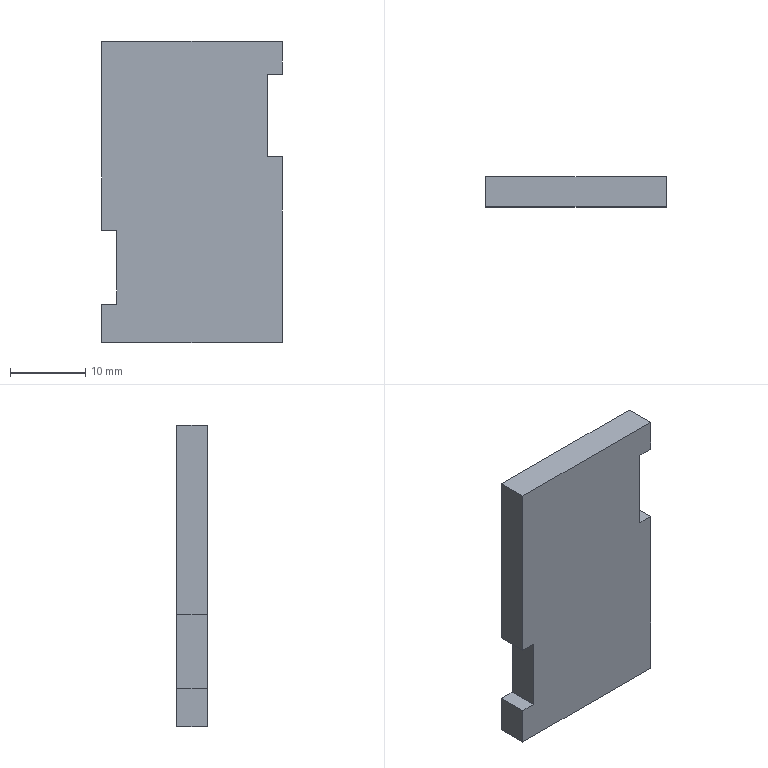Part | NX | features DATUM_CSYS 3, EXTRUDE 2, SKETCH 2 | 1 solid | 14 faces | box 24 x 4 x 40 mm | volume 3674 mm3 | plane 14
STEP:
#1=CARTESIAN_POINT('',(-12.,2.,5.103));
#2=VERTEX_POINT('',#1);
#3=CARTESIAN_POINT('',(-12.,-2.,5.103));
#4=VERTEX_POINT('',#3);
#5=CARTESIAN_POINT('',(-12.,2.,5.103));
#6=DIRECTION('',(0.,-1.,0.));
#7=VECTOR('',#6,1000.);
#8=LINE('',#5,#7);
#9=EDGE_CURVE('',#2,#4,#8,.T.);
#10=ORIENTED_EDGE('',*,*,#9,.F.);
#11=CARTESIAN_POINT('',(-12.,2.,0.));
#12=VERTEX_POINT('',#11);
#13=CARTESIAN_POINT('',(-12.,2.,40.));
#14=DIRECTION('',(0.,0.,-1.));
#15=VECTOR('',#14,1000.);
#16=LINE('',#13,#15);
#17=EDGE_CURVE('',#2,#12,#16,.T.);
#18=ORIENTED_EDGE('',*,*,#17,.T.);
#19=CARTESIAN_POINT('',(-12.,-2.,0.));
#20=VERTEX_POINT('',#19);
#21=CARTESIAN_POINT('',(-12.,2.,0.));
#22=DIRECTION('',(0.,-1.,0.));
#23=VECTOR('',#22,1000.);
#24=LINE('',#21,#23);
#25=EDGE_CURVE('',#12,#20,#24,.T.);
#26=ORIENTED_EDGE('',*,*,#25,.T.);
#27=CARTESIAN_POINT('',(-12.,-2.,40.));
#28=DIRECTION('',(0.,0.,-1.));
#29=VECTOR('',#28,1000.);
#30=LINE('',#27,#29);
#31=EDGE_CURVE('',#4,#20,#30,.T.);
#32=ORIENTED_EDGE('',*,*,#31,.F.);
#33=EDGE_LOOP('',(#10,#18,#26,#32));
#34=FACE_BOUND('',#33,.T.);
#35=CARTESIAN_POINT('',(-12.,2.,40.));
#36=DIRECTION('',(1.,0.,0.));
#37=DIRECTION('',(0.,1.,0.));
#38=AXIS2_PLACEMENT_3D('',#35,#36,#37);
#39=PLANE('',#38);
#40=ADVANCED_FACE('',(#34),#39,.F.);
#41=CARTESIAN_POINT('',(-12.,-2.,14.923));
#42=VERTEX_POINT('',#41);
#43=CARTESIAN_POINT('',(-12.,2.,14.923));
#44=VERTEX_POINT('',#43);
#45=CARTESIAN_POINT('',(-12.,2.,14.923));
#46=DIRECTION('',(0.,1.,0.));
#47=VECTOR('',#46,1000.);
#48=LINE('',#45,#47);
#49=EDGE_CURVE('',#42,#44,#48,.T.);
#50=ORIENTED_EDGE('',*,*,#49,.F.);
#51=CARTESIAN_POINT('',(-12.,-2.,40.));
#52=VERTEX_POINT('',#51);
#53=CARTESIAN_POINT('',(-12.,-2.,40.));
#54=DIRECTION('',(0.,0.,-1.));
#55=VECTOR('',#54,1000.);
#56=LINE('',#53,#55);
#57=EDGE_CURVE('',#52,#42,#56,.T.);
#58=ORIENTED_EDGE('',*,*,#57,.F.);
#59=CARTESIAN_POINT('',(-12.,2.,40.));
#60=VERTEX_POINT('',#59);
#61=CARTESIAN_POINT('',(-12.,2.,40.));
#62=DIRECTION('',(0.,-1.,0.));
#63=VECTOR('',#62,1000.);
#64=LINE('',#61,#63);
#65=EDGE_CURVE('',#60,#52,#64,.T.);
#66=ORIENTED_EDGE('',*,*,#65,.F.);
#67=CARTESIAN_POINT('',(-12.,2.,40.));
#68=DIRECTION('',(0.,0.,-1.));
#69=VECTOR('',#68,1000.);
#70=LINE('',#67,#69);
#71=EDGE_CURVE('',#60,#44,#70,.T.);
#72=ORIENTED_EDGE('',*,*,#71,.T.);
#73=EDGE_LOOP('',(#50,#58,#66,#72));
#74=FACE_BOUND('',#73,.T.);
#75=CARTESIAN_POINT('',(-12.,2.,40.));
#76=DIRECTION('',(1.,0.,0.));
#77=DIRECTION('',(0.,1.,0.));
#78=AXIS2_PLACEMENT_3D('',#75,#76,#77);
#79=PLANE('',#78);
#80=ADVANCED_FACE('',(#74),#79,.F.);
#81=CARTESIAN_POINT('',(-10.,-2.,5.103));
#82=VERTEX_POINT('',#81);
#83=CARTESIAN_POINT('',(-12.,-2.,5.103));
#84=DIRECTION('',(1.,0.,0.));
#85=VECTOR('',#84,1000.);
#86=LINE('',#83,#85);
#87=EDGE_CURVE('',#4,#82,#86,.T.);
#88=ORIENTED_EDGE('',*,*,#87,.F.);
#89=ORIENTED_EDGE('',*,*,#31,.T.);
#90=CARTESIAN_POINT('',(12.,-2.,0.));
#91=VERTEX_POINT('',#90);
#92=CARTESIAN_POINT('',(-12.,-2.,0.));
#93=DIRECTION('',(1.,0.,0.));
#94=VECTOR('',#93,1000.);
#95=LINE('',#92,#94);
#96=EDGE_CURVE('',#20,#91,#95,.T.);
#97=ORIENTED_EDGE('',*,*,#96,.T.);
#98=CARTESIAN_POINT('',(12.,-2.,24.68));
#99=VERTEX_POINT('',#98);
#100=CARTESIAN_POINT('',(12.,-2.,40.));
#101=DIRECTION('',(0.,0.,-1.));
#102=VECTOR('',#101,1000.);
#103=LINE('',#100,#102);
#104=EDGE_CURVE('',#99,#91,#103,.T.);
#105=ORIENTED_EDGE('',*,*,#104,.F.);
#106=CARTESIAN_POINT('',(9.991,-2.,24.68));
#107=VERTEX_POINT('',#106);
#108=CARTESIAN_POINT('',(-12.,-2.,24.68));
#109=DIRECTION('',(1.,0.,0.));
#110=VECTOR('',#109,1000.);
#111=LINE('',#108,#110);
#112=EDGE_CURVE('',#107,#99,#111,.T.);
#113=ORIENTED_EDGE('',*,*,#112,.F.);
#114=CARTESIAN_POINT('',(9.991,-2.,35.618));
#115=VERTEX_POINT('',#114);
#116=CARTESIAN_POINT('',(9.991,-2.,40.));
#117=DIRECTION('',(0.,0.,-1.));
#118=VECTOR('',#117,1000.);
#119=LINE('',#116,#118);
#120=EDGE_CURVE('',#115,#107,#119,.T.);
#121=ORIENTED_EDGE('',*,*,#120,.F.);
#122=CARTESIAN_POINT('',(12.,-2.,35.618));
#123=VERTEX_POINT('',#122);
#124=CARTESIAN_POINT('',(-12.,-2.,35.618));
#125=DIRECTION('',(-1.,0.,0.));
#126=VECTOR('',#125,1000.);
#127=LINE('',#124,#126);
#128=EDGE_CURVE('',#123,#115,#127,.T.);
#129=ORIENTED_EDGE('',*,*,#128,.F.);
#130=CARTESIAN_POINT('',(12.,-2.,40.));
#131=VERTEX_POINT('',#130);
#132=CARTESIAN_POINT('',(12.,-2.,40.));
#133=DIRECTION('',(0.,0.,-1.));
#134=VECTOR('',#133,1000.);
#135=LINE('',#132,#134);
#136=EDGE_CURVE('',#131,#123,#135,.T.);
#137=ORIENTED_EDGE('',*,*,#136,.F.);
#138=CARTESIAN_POINT('',(-12.,-2.,40.));
#139=DIRECTION('',(1.,0.,0.));
#140=VECTOR('',#139,1000.);
#141=LINE('',#138,#140);
#142=EDGE_CURVE('',#52,#131,#141,.T.);
#143=ORIENTED_EDGE('',*,*,#142,.F.);
#144=ORIENTED_EDGE('',*,*,#57,.T.);
#145=CARTESIAN_POINT('',(-10.,-2.,14.923));
#146=VERTEX_POINT('',#145);
#147=CARTESIAN_POINT('',(-12.,-2.,14.923));
#148=DIRECTION('',(-1.,0.,0.));
#149=VECTOR('',#148,1000.);
#150=LINE('',#147,#149);
#151=EDGE_CURVE('',#146,#42,#150,.T.);
#152=ORIENTED_EDGE('',*,*,#151,.F.);
#153=CARTESIAN_POINT('',(-10.,-2.,40.));
#154=DIRECTION('',(0.,0.,1.));
#155=VECTOR('',#154,1000.);
#156=LINE('',#153,#155);
#157=EDGE_CURVE('',#82,#146,#156,.T.);
#158=ORIENTED_EDGE('',*,*,#157,.F.);
#159=EDGE_LOOP('',(#88,#89,#97,#105,#113,#121,#129,#137,#143,#144,#152,#158));
#160=FACE_BOUND('',#159,.T.);
#161=CARTESIAN_POINT('',(-12.,-2.,40.));
#162=DIRECTION('',(0.,1.,0.));
#163=DIRECTION('',(0.,0.,1.));
#164=AXIS2_PLACEMENT_3D('',#161,#162,#163);
#165=PLANE('',#164);
#166=ADVANCED_FACE('',(#160),#165,.F.);
#167=CARTESIAN_POINT('',(12.,2.,24.68));
#168=VERTEX_POINT('',#167);
#169=CARTESIAN_POINT('',(12.,-2.,24.68));
#170=DIRECTION('',(0.,1.,0.));
#171=VECTOR('',#170,1000.);
#172=LINE('',#169,#171);
#173=EDGE_CURVE('',#99,#168,#172,.T.);
#174=ORIENTED_EDGE('',*,*,#173,.F.);
#175=ORIENTED_EDGE('',*,*,#104,.T.);
#176=CARTESIAN_POINT('',(12.,2.,0.));
#177=VERTEX_POINT('',#176);
#178=CARTESIAN_POINT('',(12.,-2.,0.));
#179=DIRECTION('',(0.,1.,0.));
#180=VECTOR('',#179,1000.);
#181=LINE('',#178,#180);
#182=EDGE_CURVE('',#91,#177,#181,.T.);
#183=ORIENTED_EDGE('',*,*,#182,.T.);
#184=CARTESIAN_POINT('',(12.,2.,40.));
#185=DIRECTION('',(0.,0.,-1.));
#186=VECTOR('',#185,1000.);
#187=LINE('',#184,#186);
#188=EDGE_CURVE('',#168,#177,#187,.T.);
#189=ORIENTED_EDGE('',*,*,#188,.F.);
#190=EDGE_LOOP('',(#174,#175,#183,#189));
#191=FACE_BOUND('',#190,.T.);
#192=CARTESIAN_POINT('',(12.,-2.,40.));
#193=DIRECTION('',(-1.,0.,0.));
#194=DIRECTION('',(0.,-1.,0.));
#195=AXIS2_PLACEMENT_3D('',#192,#193,#194);
#196=PLANE('',#195);
#197=ADVANCED_FACE('',(#191),#196,.F.);
#198=CARTESIAN_POINT('',(12.,2.,35.618));
#199=VERTEX_POINT('',#198);
#200=CARTESIAN_POINT('',(12.,-2.,35.618));
#201=DIRECTION('',(0.,-1.,0.));
#202=VECTOR('',#201,1000.);
#203=LINE('',#200,#202);
#204=EDGE_CURVE('',#199,#123,#203,.T.);
#205=ORIENTED_EDGE('',*,*,#204,.F.);
#206=CARTESIAN_POINT('',(12.,2.,40.));
#207=VERTEX_POINT('',#206);
#208=CARTESIAN_POINT('',(12.,2.,40.));
#209=DIRECTION('',(0.,0.,-1.));
#210=VECTOR('',#209,1000.);
#211=LINE('',#208,#210);
#212=EDGE_CURVE('',#207,#199,#211,.T.);
#213=ORIENTED_EDGE('',*,*,#212,.F.);
#214=CARTESIAN_POINT('',(12.,-2.,40.));
#215=DIRECTION('',(0.,1.,0.));
#216=VECTOR('',#215,1000.);
#217=LINE('',#214,#216);
#218=EDGE_CURVE('',#131,#207,#217,.T.);
#219=ORIENTED_EDGE('',*,*,#218,.F.);
#220=ORIENTED_EDGE('',*,*,#136,.T.);
#221=EDGE_LOOP('',(#205,#213,#219,#220));
#222=FACE_BOUND('',#221,.T.);
#223=CARTESIAN_POINT('',(12.,-2.,40.));
#224=DIRECTION('',(-1.,0.,0.));
#225=DIRECTION('',(0.,-1.,0.));
#226=AXIS2_PLACEMENT_3D('',#223,#224,#225);
#227=PLANE('',#226);
#228=ADVANCED_FACE('',(#222),#227,.F.);
#229=CARTESIAN_POINT('',(-10.,2.,5.103));
#230=VERTEX_POINT('',#229);
#231=CARTESIAN_POINT('',(12.,2.,5.103));
#232=DIRECTION('',(-1.,0.,0.));
#233=VECTOR('',#232,1000.);
#234=LINE('',#231,#233);
#235=EDGE_CURVE('',#230,#2,#234,.T.);
#236=ORIENTED_EDGE('',*,*,#235,.F.);
#237=CARTESIAN_POINT('',(-10.,2.,14.923));
#238=VERTEX_POINT('',#237);
#239=CARTESIAN_POINT('',(-10.,2.,40.));
#240=DIRECTION('',(0.,0.,-1.));
#241=VECTOR('',#240,1000.);
#242=LINE('',#239,#241);
#243=EDGE_CURVE('',#238,#230,#242,.T.);
#244=ORIENTED_EDGE('',*,*,#243,.F.);
#245=CARTESIAN_POINT('',(12.,2.,14.923));
#246=DIRECTION('',(1.,0.,0.));
#247=VECTOR('',#246,1000.);
#248=LINE('',#245,#247);
#249=EDGE_CURVE('',#44,#238,#248,.T.);
#250=ORIENTED_EDGE('',*,*,#249,.F.);
#251=ORIENTED_EDGE('',*,*,#71,.F.);
#252=CARTESIAN_POINT('',(12.,2.,40.));
#253=DIRECTION('',(-1.,0.,0.));
#254=VECTOR('',#253,1000.);
#255=LINE('',#252,#254);
#256=EDGE_CURVE('',#207,#60,#255,.T.);
#257=ORIENTED_EDGE('',*,*,#256,.F.);
#258=ORIENTED_EDGE('',*,*,#212,.T.);
#259=CARTESIAN_POINT('',(9.991,2.,35.618));
#260=VERTEX_POINT('',#259);
#261=CARTESIAN_POINT('',(12.,2.,35.618));
#262=DIRECTION('',(1.,0.,0.));
#263=VECTOR('',#262,1000.);
#264=LINE('',#261,#263);
#265=EDGE_CURVE('',#260,#199,#264,.T.);
#266=ORIENTED_EDGE('',*,*,#265,.F.);
#267=CARTESIAN_POINT('',(9.991,2.,24.68));
#268=VERTEX_POINT('',#267);
#269=CARTESIAN_POINT('',(9.991,2.,40.));
#270=DIRECTION('',(0.,0.,1.));
#271=VECTOR('',#270,1000.);
#272=LINE('',#269,#271);
#273=EDGE_CURVE('',#268,#260,#272,.T.);
#274=ORIENTED_EDGE('',*,*,#273,.F.);
#275=CARTESIAN_POINT('',(12.,2.,24.68));
#276=DIRECTION('',(-1.,0.,0.));
#277=VECTOR('',#276,1000.);
#278=LINE('',#275,#277);
#279=EDGE_CURVE('',#168,#268,#278,.T.);
#280=ORIENTED_EDGE('',*,*,#279,.F.);
#281=ORIENTED_EDGE('',*,*,#188,.T.);
#282=CARTESIAN_POINT('',(12.,2.,0.));
#283=DIRECTION('',(-1.,0.,0.));
#284=VECTOR('',#283,1000.);
#285=LINE('',#282,#284);
#286=EDGE_CURVE('',#177,#12,#285,.T.);
#287=ORIENTED_EDGE('',*,*,#286,.T.);
#288=ORIENTED_EDGE('',*,*,#17,.F.);
#289=EDGE_LOOP('',(#236,#244,#250,#251,#257,#258,#266,#274,#280,#281,#287,#288));
#290=FACE_BOUND('',#289,.T.);
#291=CARTESIAN_POINT('',(12.,2.,40.));
#292=DIRECTION('',(0.,-1.,0.));
#293=DIRECTION('',(0.,0.,-1.));
#294=AXIS2_PLACEMENT_3D('',#291,#292,#293);
#295=PLANE('',#294);
#296=ADVANCED_FACE('',(#290),#295,.F.);
#297=ORIENTED_EDGE('',*,*,#65,.T.);
#298=ORIENTED_EDGE('',*,*,#142,.T.);
#299=ORIENTED_EDGE('',*,*,#218,.T.);
#300=ORIENTED_EDGE('',*,*,#256,.T.);
#301=EDGE_LOOP('',(#297,#298,#299,#300));
#302=FACE_BOUND('',#301,.T.);
#303=CARTESIAN_POINT('',(0.,0.,40.));
#304=DIRECTION('',(0.,0.,1.));
#305=DIRECTION('',(1.,0.,0.));
#306=AXIS2_PLACEMENT_3D('',#303,#304,#305);
#307=PLANE('',#306);
#308=ADVANCED_FACE('',(#302),#307,.T.);
#309=ORIENTED_EDGE('',*,*,#25,.F.);
#310=ORIENTED_EDGE('',*,*,#286,.F.);
#311=ORIENTED_EDGE('',*,*,#182,.F.);
#312=ORIENTED_EDGE('',*,*,#96,.F.);
#313=EDGE_LOOP('',(#309,#310,#311,#312));
#314=FACE_BOUND('',#313,.T.);
#315=CARTESIAN_POINT('',(0.,0.,0.));
#316=DIRECTION('',(0.,0.,1.));
#317=DIRECTION('',(1.,0.,0.));
#318=AXIS2_PLACEMENT_3D('',#315,#316,#317);
#319=PLANE('',#318);
#320=ADVANCED_FACE('',(#314),#319,.F.);
#321=ORIENTED_EDGE('',*,*,#120,.T.);
#322=CARTESIAN_POINT('',(9.991,-42.,24.68));
#323=DIRECTION('',(0.,1.,0.));
#324=VECTOR('',#323,1000.);
#325=LINE('',#322,#324);
#326=EDGE_CURVE('',#268,#107,#325,.F.);
#327=ORIENTED_EDGE('',*,*,#326,.F.);
#328=ORIENTED_EDGE('',*,*,#273,.T.);
#329=CARTESIAN_POINT('',(9.991,-42.,35.618));
#330=DIRECTION('',(0.,1.,0.));
#331=VECTOR('',#330,1000.);
#332=LINE('',#329,#331);
#333=EDGE_CURVE('',#260,#115,#332,.F.);
#334=ORIENTED_EDGE('',*,*,#333,.T.);
#335=EDGE_LOOP('',(#321,#327,#328,#334));
#336=FACE_BOUND('',#335,.T.);
#337=CARTESIAN_POINT('',(9.991,-42.,35.618));
#338=DIRECTION('',(1.,0.,0.));
#339=DIRECTION('',(0.,0.,-1.));
#340=AXIS2_PLACEMENT_3D('',#337,#338,#339);
#341=PLANE('',#340);
#342=ADVANCED_FACE('',(#336),#341,.T.);
#343=ORIENTED_EDGE('',*,*,#112,.T.);
#344=ORIENTED_EDGE('',*,*,#173,.T.);
#345=ORIENTED_EDGE('',*,*,#279,.T.);
#346=ORIENTED_EDGE('',*,*,#326,.T.);
#347=EDGE_LOOP('',(#343,#344,#345,#346));
#348=FACE_BOUND('',#347,.T.);
#349=CARTESIAN_POINT('',(9.991,-42.,24.68));
#350=DIRECTION('',(0.,0.,1.));
#351=DIRECTION('',(1.,0.,0.));
#352=AXIS2_PLACEMENT_3D('',#349,#350,#351);
#353=PLANE('',#352);
#354=ADVANCED_FACE('',(#348),#353,.T.);
#355=ORIENTED_EDGE('',*,*,#128,.T.);
#356=ORIENTED_EDGE('',*,*,#333,.F.);
#357=ORIENTED_EDGE('',*,*,#265,.T.);
#358=ORIENTED_EDGE('',*,*,#204,.T.);
#359=EDGE_LOOP('',(#355,#356,#357,#358));
#360=FACE_BOUND('',#359,.T.);
#361=CARTESIAN_POINT('',(14.009,-42.,35.618));
#362=DIRECTION('',(0.,0.,-1.));
#363=DIRECTION('',(-1.,0.,0.));
#364=AXIS2_PLACEMENT_3D('',#361,#362,#363);
#365=PLANE('',#364);
#366=ADVANCED_FACE('',(#360),#365,.T.);
#367=ORIENTED_EDGE('',*,*,#87,.T.);
#368=CARTESIAN_POINT('',(-10.,-42.,5.103));
#369=DIRECTION('',(0.,1.,0.));
#370=VECTOR('',#369,1000.);
#371=LINE('',#368,#370);
#372=EDGE_CURVE('',#230,#82,#371,.F.);
#373=ORIENTED_EDGE('',*,*,#372,.F.);
#374=ORIENTED_EDGE('',*,*,#235,.T.);
#375=ORIENTED_EDGE('',*,*,#9,.T.);
#376=EDGE_LOOP('',(#367,#373,#374,#375));
#377=FACE_BOUND('',#376,.T.);
#378=CARTESIAN_POINT('',(-14.,-42.,5.103));
#379=DIRECTION('',(0.,0.,1.));
#380=DIRECTION('',(1.,0.,0.));
#381=AXIS2_PLACEMENT_3D('',#378,#379,#380);
#382=PLANE('',#381);
#383=ADVANCED_FACE('',(#377),#382,.T.);
#384=ORIENTED_EDGE('',*,*,#157,.T.);
#385=CARTESIAN_POINT('',(-10.,-42.,14.923));
#386=DIRECTION('',(0.,1.,0.));
#387=VECTOR('',#386,1000.);
#388=LINE('',#385,#387);
#389=EDGE_CURVE('',#238,#146,#388,.F.);
#390=ORIENTED_EDGE('',*,*,#389,.F.);
#391=ORIENTED_EDGE('',*,*,#243,.T.);
#392=ORIENTED_EDGE('',*,*,#372,.T.);
#393=EDGE_LOOP('',(#384,#390,#391,#392));
#394=FACE_BOUND('',#393,.T.);
#395=CARTESIAN_POINT('',(-10.,-42.,5.103));
#396=DIRECTION('',(-1.,0.,0.));
#397=DIRECTION('',(0.,0.,1.));
#398=AXIS2_PLACEMENT_3D('',#395,#396,#397);
#399=PLANE('',#398);
#400=ADVANCED_FACE('',(#394),#399,.T.);
#401=ORIENTED_EDGE('',*,*,#151,.T.);
#402=ORIENTED_EDGE('',*,*,#49,.T.);
#403=ORIENTED_EDGE('',*,*,#249,.T.);
#404=ORIENTED_EDGE('',*,*,#389,.T.);
#405=EDGE_LOOP('',(#401,#402,#403,#404));
#406=FACE_BOUND('',#405,.T.);
#407=CARTESIAN_POINT('',(-10.,-42.,14.923));
#408=DIRECTION('',(0.,0.,-1.));
#409=DIRECTION('',(-1.,0.,0.));
#410=AXIS2_PLACEMENT_3D('',#407,#408,#409);
#411=PLANE('',#410);
#412=ADVANCED_FACE('',(#406),#411,.T.);
#413=CLOSED_SHELL('',(#40,#80,#166,#197,#228,#296,#308,#320,#342,#354,#366,#383,#400,#412));
#414=MANIFOLD_SOLID_BREP('',#413);
#415=(LENGTH_UNIT()NAMED_UNIT(*)SI_UNIT(.MILLI.,.METRE.));
#416=UNCERTAINTY_MEASURE_WITH_UNIT(LENGTH_MEASURE(0.00001),#415,'','');
#417=(NAMED_UNIT(*)PLANE_ANGLE_UNIT()SI_UNIT($,.RADIAN.));
#418=(NAMED_UNIT(*)SI_UNIT($,.STERADIAN.)SOLID_ANGLE_UNIT());
#419=(GEOMETRIC_REPRESENTATION_CONTEXT(3)GLOBAL_UNCERTAINTY_ASSIGNED_CONTEXT((#416))GLOBAL_UNIT_ASSIGNED_CONTEXT((#415,#417,#418))REPRESENTATION_CONTEXT('',''));
#420=ADVANCED_BREP_SHAPE_REPRESENTATION('',(#414),#419);